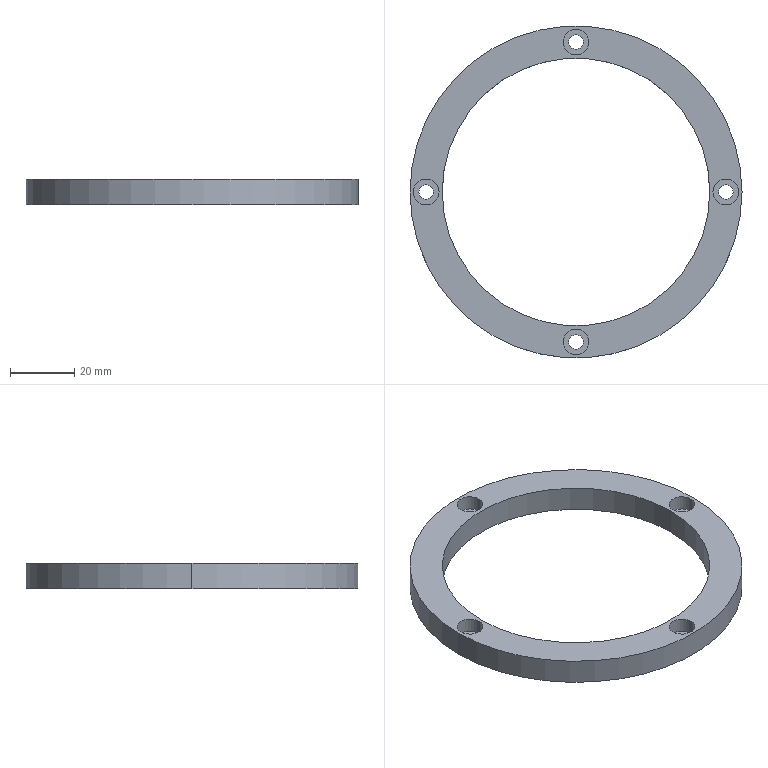Part | SolidWorks | features CirPattern 1, Extrusion 1, HoleWzd 1 | 1 solid | 26 faces | box 103 x 103 x 8 mm | volume 22232 mm3 | cylinder 20 | plane 6 | commonest cylinder face diameters 4.5 x8 8 x8 83 x2 103 x2
STEP:
#1=CARTESIAN_POINT('',(-50.5,0.,3.4));
#2=VERTEX_POINT('',#1);
#3=CARTESIAN_POINT('',(-42.5,0.,3.4));
#4=VERTEX_POINT('',#3);
#5=CARTESIAN_POINT('',(-46.5,0.,3.4));
#6=DIRECTION('',(0.,0.,1.));
#7=DIRECTION('',(1.,0.,0.));
#8=AXIS2_PLACEMENT_3D('',#5,#6,#7);
#9=CIRCLE('',#8,4.);
#10=EDGE_CURVE('',#2,#4,#9,.T.);
#11=ORIENTED_EDGE('',*,*,#10,.F.);
#12=CARTESIAN_POINT('',(-50.5,0.,8.));
#13=VERTEX_POINT('',#12);
#14=CARTESIAN_POINT('',(-50.5,0.,8.));
#15=DIRECTION('',(0.,0.,1.));
#16=VECTOR('',#15,1000.);
#17=LINE('',#14,#16);
#18=EDGE_CURVE('',#2,#13,#17,.T.);
#19=ORIENTED_EDGE('',*,*,#18,.T.);
#20=CARTESIAN_POINT('',(-42.5,0.,8.));
#21=VERTEX_POINT('',#20);
#22=CARTESIAN_POINT('',(-46.5,0.,8.));
#23=DIRECTION('',(0.,0.,1.));
#24=DIRECTION('',(1.,0.,0.));
#25=AXIS2_PLACEMENT_3D('',#22,#23,#24);
#26=CIRCLE('',#25,4.);
#27=EDGE_CURVE('',#13,#21,#26,.T.);
#28=ORIENTED_EDGE('',*,*,#27,.T.);
#29=CARTESIAN_POINT('',(-42.5,0.,8.));
#30=DIRECTION('',(0.,0.,1.));
#31=VECTOR('',#30,1000.);
#32=LINE('',#29,#31);
#33=EDGE_CURVE('',#4,#21,#32,.T.);
#34=ORIENTED_EDGE('',*,*,#33,.F.);
#35=EDGE_LOOP('',(#11,#19,#28,#34));
#36=FACE_OUTER_BOUND('',#35,.T.);
#37=CARTESIAN_POINT('',(-46.5,0.,8.));
#38=DIRECTION('',(0.,0.,1.));
#39=DIRECTION('',(1.,0.,0.));
#40=AXIS2_PLACEMENT_3D('',#37,#38,#39);
#41=CYLINDRICAL_SURFACE('',#40,4.);
#42=ADVANCED_FACE('',(#36),#41,.F.);
#43=CARTESIAN_POINT('',(-48.75,0.,0.));
#44=VERTEX_POINT('',#43);
#45=CARTESIAN_POINT('',(-44.25,0.,0.));
#46=VERTEX_POINT('',#45);
#47=CARTESIAN_POINT('',(-46.5,0.,0.));
#48=DIRECTION('',(0.,0.,1.));
#49=DIRECTION('',(1.,0.,0.));
#50=AXIS2_PLACEMENT_3D('',#47,#48,#49);
#51=CIRCLE('',#50,2.25);
#52=EDGE_CURVE('',#44,#46,#51,.T.);
#53=ORIENTED_EDGE('',*,*,#52,.F.);
#54=CARTESIAN_POINT('',(-48.75,0.,3.4));
#55=VERTEX_POINT('',#54);
#56=CARTESIAN_POINT('',(-48.75,0.,8.));
#57=DIRECTION('',(0.,0.,1.));
#58=VECTOR('',#57,1000.);
#59=LINE('',#56,#58);
#60=EDGE_CURVE('',#44,#55,#59,.T.);
#61=ORIENTED_EDGE('',*,*,#60,.T.);
#62=CARTESIAN_POINT('',(-44.25,0.,3.4));
#63=VERTEX_POINT('',#62);
#64=CARTESIAN_POINT('',(-46.5,0.,3.4));
#65=DIRECTION('',(0.,0.,1.));
#66=DIRECTION('',(1.,0.,0.));
#67=AXIS2_PLACEMENT_3D('',#64,#65,#66);
#68=CIRCLE('',#67,2.25);
#69=EDGE_CURVE('',#55,#63,#68,.T.);
#70=ORIENTED_EDGE('',*,*,#69,.T.);
#71=CARTESIAN_POINT('',(-44.25,0.,8.));
#72=DIRECTION('',(0.,0.,1.));
#73=VECTOR('',#72,1000.);
#74=LINE('',#71,#73);
#75=EDGE_CURVE('',#46,#63,#74,.T.);
#76=ORIENTED_EDGE('',*,*,#75,.F.);
#77=EDGE_LOOP('',(#53,#61,#70,#76));
#78=FACE_OUTER_BOUND('',#77,.T.);
#79=CARTESIAN_POINT('',(-46.5,0.,8.));
#80=DIRECTION('',(0.,0.,1.));
#81=DIRECTION('',(1.,0.,0.));
#82=AXIS2_PLACEMENT_3D('',#79,#80,#81);
#83=CYLINDRICAL_SURFACE('',#82,2.25);
#84=ADVANCED_FACE('',(#78),#83,.F.);
#85=CARTESIAN_POINT('',(-4.,-46.5,3.4));
#86=VERTEX_POINT('',#85);
#87=CARTESIAN_POINT('',(4.,-46.5,3.4));
#88=VERTEX_POINT('',#87);
#89=CARTESIAN_POINT('',(0.,-46.5,3.4));
#90=DIRECTION('',(0.,0.,1.));
#91=DIRECTION('',(1.,0.,0.));
#92=AXIS2_PLACEMENT_3D('',#89,#90,#91);
#93=CIRCLE('',#92,4.);
#94=EDGE_CURVE('',#86,#88,#93,.T.);
#95=ORIENTED_EDGE('',*,*,#94,.F.);
#96=CARTESIAN_POINT('',(-4.,-46.5,8.));
#97=VERTEX_POINT('',#96);
#98=CARTESIAN_POINT('',(-4.,-46.5,8.));
#99=DIRECTION('',(0.,0.,1.));
#100=VECTOR('',#99,1000.);
#101=LINE('',#98,#100);
#102=EDGE_CURVE('',#86,#97,#101,.T.);
#103=ORIENTED_EDGE('',*,*,#102,.T.);
#104=CARTESIAN_POINT('',(4.,-46.5,8.));
#105=VERTEX_POINT('',#104);
#106=CARTESIAN_POINT('',(0.,-46.5,8.));
#107=DIRECTION('',(0.,0.,1.));
#108=DIRECTION('',(1.,0.,0.));
#109=AXIS2_PLACEMENT_3D('',#106,#107,#108);
#110=CIRCLE('',#109,4.);
#111=EDGE_CURVE('',#97,#105,#110,.T.);
#112=ORIENTED_EDGE('',*,*,#111,.T.);
#113=CARTESIAN_POINT('',(4.,-46.5,8.));
#114=DIRECTION('',(0.,0.,1.));
#115=VECTOR('',#114,1000.);
#116=LINE('',#113,#115);
#117=EDGE_CURVE('',#88,#105,#116,.T.);
#118=ORIENTED_EDGE('',*,*,#117,.F.);
#119=EDGE_LOOP('',(#95,#103,#112,#118));
#120=FACE_OUTER_BOUND('',#119,.T.);
#121=CARTESIAN_POINT('',(0.,-46.5,8.));
#122=DIRECTION('',(0.,0.,1.));
#123=DIRECTION('',(1.,0.,0.));
#124=AXIS2_PLACEMENT_3D('',#121,#122,#123);
#125=CYLINDRICAL_SURFACE('',#124,4.);
#126=ADVANCED_FACE('',(#120),#125,.F.);
#127=CARTESIAN_POINT('',(-2.25,-46.5,0.));
#128=VERTEX_POINT('',#127);
#129=CARTESIAN_POINT('',(2.25,-46.5,0.));
#130=VERTEX_POINT('',#129);
#131=CARTESIAN_POINT('',(0.,-46.5,0.));
#132=DIRECTION('',(0.,0.,1.));
#133=DIRECTION('',(1.,0.,0.));
#134=AXIS2_PLACEMENT_3D('',#131,#132,#133);
#135=CIRCLE('',#134,2.25);
#136=EDGE_CURVE('',#128,#130,#135,.T.);
#137=ORIENTED_EDGE('',*,*,#136,.F.);
#138=CARTESIAN_POINT('',(-2.25,-46.5,3.4));
#139=VERTEX_POINT('',#138);
#140=CARTESIAN_POINT('',(-2.25,-46.5,8.));
#141=DIRECTION('',(0.,0.,1.));
#142=VECTOR('',#141,1000.);
#143=LINE('',#140,#142);
#144=EDGE_CURVE('',#128,#139,#143,.T.);
#145=ORIENTED_EDGE('',*,*,#144,.T.);
#146=CARTESIAN_POINT('',(2.25,-46.5,3.4));
#147=VERTEX_POINT('',#146);
#148=CARTESIAN_POINT('',(0.,-46.5,3.4));
#149=DIRECTION('',(0.,0.,1.));
#150=DIRECTION('',(1.,0.,0.));
#151=AXIS2_PLACEMENT_3D('',#148,#149,#150);
#152=CIRCLE('',#151,2.25);
#153=EDGE_CURVE('',#139,#147,#152,.T.);
#154=ORIENTED_EDGE('',*,*,#153,.T.);
#155=CARTESIAN_POINT('',(2.25,-46.5,8.));
#156=DIRECTION('',(0.,0.,1.));
#157=VECTOR('',#156,1000.);
#158=LINE('',#155,#157);
#159=EDGE_CURVE('',#130,#147,#158,.T.);
#160=ORIENTED_EDGE('',*,*,#159,.F.);
#161=EDGE_LOOP('',(#137,#145,#154,#160));
#162=FACE_OUTER_BOUND('',#161,.T.);
#163=CARTESIAN_POINT('',(0.,-46.5,8.));
#164=DIRECTION('',(0.,0.,1.));
#165=DIRECTION('',(1.,0.,0.));
#166=AXIS2_PLACEMENT_3D('',#163,#164,#165);
#167=CYLINDRICAL_SURFACE('',#166,2.25);
#168=ADVANCED_FACE('',(#162),#167,.F.);
#169=CARTESIAN_POINT('',(42.5,0.,3.4));
#170=VERTEX_POINT('',#169);
#171=CARTESIAN_POINT('',(50.5,0.,3.4));
#172=VERTEX_POINT('',#171);
#173=CARTESIAN_POINT('',(46.5,0.,3.4));
#174=DIRECTION('',(0.,0.,1.));
#175=DIRECTION('',(1.,0.,0.));
#176=AXIS2_PLACEMENT_3D('',#173,#174,#175);
#177=CIRCLE('',#176,4.);
#178=EDGE_CURVE('',#170,#172,#177,.T.);
#179=ORIENTED_EDGE('',*,*,#178,.F.);
#180=CARTESIAN_POINT('',(42.5,0.,8.));
#181=VERTEX_POINT('',#180);
#182=CARTESIAN_POINT('',(42.5,0.,8.));
#183=DIRECTION('',(0.,0.,1.));
#184=VECTOR('',#183,1000.);
#185=LINE('',#182,#184);
#186=EDGE_CURVE('',#170,#181,#185,.T.);
#187=ORIENTED_EDGE('',*,*,#186,.T.);
#188=CARTESIAN_POINT('',(50.5,0.,8.));
#189=VERTEX_POINT('',#188);
#190=CARTESIAN_POINT('',(46.5,0.,8.));
#191=DIRECTION('',(0.,0.,1.));
#192=DIRECTION('',(1.,0.,0.));
#193=AXIS2_PLACEMENT_3D('',#190,#191,#192);
#194=CIRCLE('',#193,4.);
#195=EDGE_CURVE('',#181,#189,#194,.T.);
#196=ORIENTED_EDGE('',*,*,#195,.T.);
#197=CARTESIAN_POINT('',(50.5,0.,8.));
#198=DIRECTION('',(0.,0.,1.));
#199=VECTOR('',#198,1000.);
#200=LINE('',#197,#199);
#201=EDGE_CURVE('',#172,#189,#200,.T.);
#202=ORIENTED_EDGE('',*,*,#201,.F.);
#203=EDGE_LOOP('',(#179,#187,#196,#202));
#204=FACE_OUTER_BOUND('',#203,.T.);
#205=CARTESIAN_POINT('',(46.5,0.,8.));
#206=DIRECTION('',(0.,0.,1.));
#207=DIRECTION('',(1.,0.,0.));
#208=AXIS2_PLACEMENT_3D('',#205,#206,#207);
#209=CYLINDRICAL_SURFACE('',#208,4.);
#210=ADVANCED_FACE('',(#204),#209,.F.);
#211=CARTESIAN_POINT('',(44.25,0.,0.));
#212=VERTEX_POINT('',#211);
#213=CARTESIAN_POINT('',(48.75,0.,0.));
#214=VERTEX_POINT('',#213);
#215=CARTESIAN_POINT('',(46.5,0.,0.));
#216=DIRECTION('',(0.,0.,1.));
#217=DIRECTION('',(1.,0.,0.));
#218=AXIS2_PLACEMENT_3D('',#215,#216,#217);
#219=CIRCLE('',#218,2.25);
#220=EDGE_CURVE('',#212,#214,#219,.T.);
#221=ORIENTED_EDGE('',*,*,#220,.F.);
#222=CARTESIAN_POINT('',(44.25,0.,3.4));
#223=VERTEX_POINT('',#222);
#224=CARTESIAN_POINT('',(44.25,0.,8.));
#225=DIRECTION('',(0.,0.,1.));
#226=VECTOR('',#225,1000.);
#227=LINE('',#224,#226);
#228=EDGE_CURVE('',#212,#223,#227,.T.);
#229=ORIENTED_EDGE('',*,*,#228,.T.);
#230=CARTESIAN_POINT('',(48.75,0.,3.4));
#231=VERTEX_POINT('',#230);
#232=CARTESIAN_POINT('',(46.5,0.,3.4));
#233=DIRECTION('',(0.,0.,1.));
#234=DIRECTION('',(1.,0.,0.));
#235=AXIS2_PLACEMENT_3D('',#232,#233,#234);
#236=CIRCLE('',#235,2.25);
#237=EDGE_CURVE('',#223,#231,#236,.T.);
#238=ORIENTED_EDGE('',*,*,#237,.T.);
#239=CARTESIAN_POINT('',(48.75,0.,8.));
#240=DIRECTION('',(0.,0.,1.));
#241=VECTOR('',#240,1000.);
#242=LINE('',#239,#241);
#243=EDGE_CURVE('',#214,#231,#242,.T.);
#244=ORIENTED_EDGE('',*,*,#243,.F.);
#245=EDGE_LOOP('',(#221,#229,#238,#244));
#246=FACE_OUTER_BOUND('',#245,.T.);
#247=CARTESIAN_POINT('',(46.5,0.,8.));
#248=DIRECTION('',(0.,0.,1.));
#249=DIRECTION('',(1.,0.,0.));
#250=AXIS2_PLACEMENT_3D('',#247,#248,#249);
#251=CYLINDRICAL_SURFACE('',#250,2.25);
#252=ADVANCED_FACE('',(#246),#251,.F.);
#253=CARTESIAN_POINT('',(-4.,46.5,3.4));
#254=VERTEX_POINT('',#253);
#255=CARTESIAN_POINT('',(4.,46.5,3.4));
#256=VERTEX_POINT('',#255);
#257=CARTESIAN_POINT('',(0.,46.5,3.4));
#258=DIRECTION('',(0.,0.,1.));
#259=DIRECTION('',(1.,0.,0.));
#260=AXIS2_PLACEMENT_3D('',#257,#258,#259);
#261=CIRCLE('',#260,4.);
#262=EDGE_CURVE('',#254,#256,#261,.T.);
#263=ORIENTED_EDGE('',*,*,#262,.F.);
#264=CARTESIAN_POINT('',(-4.,46.5,8.));
#265=VERTEX_POINT('',#264);
#266=CARTESIAN_POINT('',(-4.,46.5,8.));
#267=DIRECTION('',(0.,0.,1.));
#268=VECTOR('',#267,1000.);
#269=LINE('',#266,#268);
#270=EDGE_CURVE('',#254,#265,#269,.T.);
#271=ORIENTED_EDGE('',*,*,#270,.T.);
#272=CARTESIAN_POINT('',(4.,46.5,8.));
#273=VERTEX_POINT('',#272);
#274=CARTESIAN_POINT('',(0.,46.5,8.));
#275=DIRECTION('',(0.,0.,1.));
#276=DIRECTION('',(1.,0.,0.));
#277=AXIS2_PLACEMENT_3D('',#274,#275,#276);
#278=CIRCLE('',#277,4.);
#279=EDGE_CURVE('',#265,#273,#278,.T.);
#280=ORIENTED_EDGE('',*,*,#279,.T.);
#281=CARTESIAN_POINT('',(4.,46.5,8.));
#282=DIRECTION('',(0.,0.,1.));
#283=VECTOR('',#282,1000.);
#284=LINE('',#281,#283);
#285=EDGE_CURVE('',#256,#273,#284,.T.);
#286=ORIENTED_EDGE('',*,*,#285,.F.);
#287=EDGE_LOOP('',(#263,#271,#280,#286));
#288=FACE_OUTER_BOUND('',#287,.T.);
#289=CARTESIAN_POINT('',(0.,46.5,8.));
#290=DIRECTION('',(0.,0.,1.));
#291=DIRECTION('',(1.,0.,0.));
#292=AXIS2_PLACEMENT_3D('',#289,#290,#291);
#293=CYLINDRICAL_SURFACE('',#292,4.);
#294=ADVANCED_FACE('',(#288),#293,.F.);
#295=CARTESIAN_POINT('',(-2.25,46.5,0.));
#296=VERTEX_POINT('',#295);
#297=CARTESIAN_POINT('',(2.25,46.5,0.));
#298=VERTEX_POINT('',#297);
#299=CARTESIAN_POINT('',(0.,46.5,0.));
#300=DIRECTION('',(0.,0.,1.));
#301=DIRECTION('',(1.,0.,0.));
#302=AXIS2_PLACEMENT_3D('',#299,#300,#301);
#303=CIRCLE('',#302,2.25);
#304=EDGE_CURVE('',#296,#298,#303,.T.);
#305=ORIENTED_EDGE('',*,*,#304,.F.);
#306=CARTESIAN_POINT('',(-2.25,46.5,3.4));
#307=VERTEX_POINT('',#306);
#308=CARTESIAN_POINT('',(-2.25,46.5,8.));
#309=DIRECTION('',(0.,0.,1.));
#310=VECTOR('',#309,1000.);
#311=LINE('',#308,#310);
#312=EDGE_CURVE('',#296,#307,#311,.T.);
#313=ORIENTED_EDGE('',*,*,#312,.T.);
#314=CARTESIAN_POINT('',(2.25,46.5,3.4));
#315=VERTEX_POINT('',#314);
#316=CARTESIAN_POINT('',(0.,46.5,3.4));
#317=DIRECTION('',(0.,0.,1.));
#318=DIRECTION('',(1.,0.,0.));
#319=AXIS2_PLACEMENT_3D('',#316,#317,#318);
#320=CIRCLE('',#319,2.25);
#321=EDGE_CURVE('',#307,#315,#320,.T.);
#322=ORIENTED_EDGE('',*,*,#321,.T.);
#323=CARTESIAN_POINT('',(2.25,46.5,8.));
#324=DIRECTION('',(0.,0.,1.));
#325=VECTOR('',#324,1000.);
#326=LINE('',#323,#325);
#327=EDGE_CURVE('',#298,#315,#326,.T.);
#328=ORIENTED_EDGE('',*,*,#327,.F.);
#329=EDGE_LOOP('',(#305,#313,#322,#328));
#330=FACE_OUTER_BOUND('',#329,.T.);
#331=CARTESIAN_POINT('',(0.,46.5,8.));
#332=DIRECTION('',(0.,0.,1.));
#333=DIRECTION('',(1.,0.,0.));
#334=AXIS2_PLACEMENT_3D('',#331,#332,#333);
#335=CYLINDRICAL_SURFACE('',#334,2.25);
#336=ADVANCED_FACE('',(#330),#335,.F.);
#337=CARTESIAN_POINT('',(-41.5,0.,8.));
#338=VERTEX_POINT('',#337);
#339=CARTESIAN_POINT('',(41.5,0.,8.));
#340=VERTEX_POINT('',#339);
#341=CARTESIAN_POINT('',(0.,0.,8.));
#342=DIRECTION('',(0.,0.,1.));
#343=DIRECTION('',(1.,0.,0.));
#344=AXIS2_PLACEMENT_3D('',#341,#342,#343);
#345=CIRCLE('',#344,41.5);
#346=EDGE_CURVE('',#338,#340,#345,.T.);
#347=ORIENTED_EDGE('',*,*,#346,.T.);
#348=CARTESIAN_POINT('',(41.5,0.,0.));
#349=VERTEX_POINT('',#348);
#350=CARTESIAN_POINT('',(41.5,0.,8.));
#351=DIRECTION('',(0.,0.,-1.));
#352=VECTOR('',#351,1000.);
#353=LINE('',#350,#352);
#354=EDGE_CURVE('',#340,#349,#353,.T.);
#355=ORIENTED_EDGE('',*,*,#354,.T.);
#356=CARTESIAN_POINT('',(-41.5,0.,0.));
#357=VERTEX_POINT('',#356);
#358=CARTESIAN_POINT('',(0.,0.,0.));
#359=DIRECTION('',(0.,0.,1.));
#360=DIRECTION('',(1.,0.,0.));
#361=AXIS2_PLACEMENT_3D('',#358,#359,#360);
#362=CIRCLE('',#361,41.5);
#363=EDGE_CURVE('',#357,#349,#362,.T.);
#364=ORIENTED_EDGE('',*,*,#363,.F.);
#365=CARTESIAN_POINT('',(-41.5,0.,8.));
#366=DIRECTION('',(0.,0.,-1.));
#367=VECTOR('',#366,1000.);
#368=LINE('',#365,#367);
#369=EDGE_CURVE('',#338,#357,#368,.T.);
#370=ORIENTED_EDGE('',*,*,#369,.F.);
#371=EDGE_LOOP('',(#347,#355,#364,#370));
#372=FACE_OUTER_BOUND('',#371,.T.);
#373=CARTESIAN_POINT('',(0.,0.,8.));
#374=DIRECTION('',(0.,0.,-1.));
#375=DIRECTION('',(-1.,0.,0.));
#376=AXIS2_PLACEMENT_3D('',#373,#374,#375);
#377=CYLINDRICAL_SURFACE('',#376,41.5);
#378=ADVANCED_FACE('',(#372),#377,.F.);
#379=CARTESIAN_POINT('',(51.5,0.,8.));
#380=VERTEX_POINT('',#379);
#381=CARTESIAN_POINT('',(-51.5,0.,8.));
#382=VERTEX_POINT('',#381);
#383=CARTESIAN_POINT('',(0.,0.,8.));
#384=DIRECTION('',(0.,0.,1.));
#385=DIRECTION('',(1.,0.,0.));
#386=AXIS2_PLACEMENT_3D('',#383,#384,#385);
#387=CIRCLE('',#386,51.5);
#388=EDGE_CURVE('',#380,#382,#387,.T.);
#389=ORIENTED_EDGE('',*,*,#388,.F.);
#390=CARTESIAN_POINT('',(51.5,0.,0.));
#391=VERTEX_POINT('',#390);
#392=CARTESIAN_POINT('',(51.5,0.,8.));
#393=DIRECTION('',(0.,0.,-1.));
#394=VECTOR('',#393,1000.);
#395=LINE('',#392,#394);
#396=EDGE_CURVE('',#380,#391,#395,.T.);
#397=ORIENTED_EDGE('',*,*,#396,.T.);
#398=CARTESIAN_POINT('',(-51.5,0.,0.));
#399=VERTEX_POINT('',#398);
#400=CARTESIAN_POINT('',(0.,0.,0.));
#401=DIRECTION('',(0.,0.,1.));
#402=DIRECTION('',(1.,0.,0.));
#403=AXIS2_PLACEMENT_3D('',#400,#401,#402);
#404=CIRCLE('',#403,51.5);
#405=EDGE_CURVE('',#391,#399,#404,.T.);
#406=ORIENTED_EDGE('',*,*,#405,.T.);
#407=CARTESIAN_POINT('',(-51.5,0.,8.));
#408=DIRECTION('',(0.,0.,-1.));
#409=VECTOR('',#408,1000.);
#410=LINE('',#407,#409);
#411=EDGE_CURVE('',#382,#399,#410,.T.);
#412=ORIENTED_EDGE('',*,*,#411,.F.);
#413=EDGE_LOOP('',(#389,#397,#406,#412));
#414=FACE_OUTER_BOUND('',#413,.T.);
#415=CARTESIAN_POINT('',(0.,0.,8.));
#416=DIRECTION('',(0.,0.,-1.));
#417=DIRECTION('',(-1.,0.,0.));
#418=AXIS2_PLACEMENT_3D('',#415,#416,#417);
#419=CYLINDRICAL_SURFACE('',#418,51.5);
#420=ADVANCED_FACE('',(#414),#419,.T.);
#421=CARTESIAN_POINT('',(-46.5,0.,8.));
#422=DIRECTION('',(0.,0.,1.));
#423=DIRECTION('',(1.,0.,0.));
#424=AXIS2_PLACEMENT_3D('',#421,#422,#423);
#425=CIRCLE('',#424,4.);
#426=EDGE_CURVE('',#21,#13,#425,.T.);
#427=ORIENTED_EDGE('',*,*,#426,.F.);
#428=ORIENTED_EDGE('',*,*,#27,.F.);
#429=EDGE_LOOP('',(#427,#428));
#430=FACE_BOUND('',#429,.T.);
#431=CARTESIAN_POINT('',(0.,-46.5,8.));
#432=DIRECTION('',(0.,0.,1.));
#433=DIRECTION('',(1.,0.,0.));
#434=AXIS2_PLACEMENT_3D('',#431,#432,#433);
#435=CIRCLE('',#434,4.);
#436=EDGE_CURVE('',#105,#97,#435,.T.);
#437=ORIENTED_EDGE('',*,*,#436,.F.);
#438=ORIENTED_EDGE('',*,*,#111,.F.);
#439=EDGE_LOOP('',(#437,#438));
#440=FACE_BOUND('',#439,.T.);
#441=CARTESIAN_POINT('',(46.5,0.,8.));
#442=DIRECTION('',(0.,0.,1.));
#443=DIRECTION('',(1.,0.,0.));
#444=AXIS2_PLACEMENT_3D('',#441,#442,#443);
#445=CIRCLE('',#444,4.);
#446=EDGE_CURVE('',#189,#181,#445,.T.);
#447=ORIENTED_EDGE('',*,*,#446,.F.);
#448=ORIENTED_EDGE('',*,*,#195,.F.);
#449=EDGE_LOOP('',(#447,#448));
#450=FACE_BOUND('',#449,.T.);
#451=CARTESIAN_POINT('',(0.,46.5,8.));
#452=DIRECTION('',(0.,0.,1.));
#453=DIRECTION('',(1.,0.,0.));
#454=AXIS2_PLACEMENT_3D('',#451,#452,#453);
#455=CIRCLE('',#454,4.);
#456=EDGE_CURVE('',#273,#265,#455,.T.);
#457=ORIENTED_EDGE('',*,*,#456,.F.);
#458=ORIENTED_EDGE('',*,*,#279,.F.);
#459=EDGE_LOOP('',(#457,#458));
#460=FACE_BOUND('',#459,.T.);
#461=CARTESIAN_POINT('',(0.,0.,8.));
#462=DIRECTION('',(0.,0.,1.));
#463=DIRECTION('',(1.,0.,0.));
#464=AXIS2_PLACEMENT_3D('',#461,#462,#463);
#465=CIRCLE('',#464,51.5);
#466=EDGE_CURVE('',#382,#380,#465,.T.);
#467=ORIENTED_EDGE('',*,*,#466,.T.);
#468=ORIENTED_EDGE('',*,*,#388,.T.);
#469=EDGE_LOOP('',(#467,#468));
#470=FACE_OUTER_BOUND('',#469,.T.);
#471=ORIENTED_EDGE('',*,*,#346,.F.);
#472=CARTESIAN_POINT('',(0.,0.,8.));
#473=DIRECTION('',(0.,0.,1.));
#474=DIRECTION('',(1.,0.,0.));
#475=AXIS2_PLACEMENT_3D('',#472,#473,#474);
#476=CIRCLE('',#475,41.5);
#477=EDGE_CURVE('',#340,#338,#476,.T.);
#478=ORIENTED_EDGE('',*,*,#477,.F.);
#479=EDGE_LOOP('',(#471,#478));
#480=FACE_BOUND('',#479,.T.);
#481=CARTESIAN_POINT('',(0.,0.,8.));
#482=DIRECTION('',(0.,0.,1.));
#483=DIRECTION('',(1.,0.,0.));
#484=AXIS2_PLACEMENT_3D('',#481,#482,#483);
#485=PLANE('',#484);
#486=ADVANCED_FACE('',(#430,#440,#450,#460,#470,#480),#485,.T.);
#487=CARTESIAN_POINT('',(-46.5,0.,0.));
#488=DIRECTION('',(0.,0.,1.));
#489=DIRECTION('',(1.,0.,0.));
#490=AXIS2_PLACEMENT_3D('',#487,#488,#489);
#491=CIRCLE('',#490,2.25);
#492=EDGE_CURVE('',#46,#44,#491,.T.);
#493=ORIENTED_EDGE('',*,*,#492,.T.);
#494=ORIENTED_EDGE('',*,*,#52,.T.);
#495=EDGE_LOOP('',(#493,#494));
#496=FACE_BOUND('',#495,.T.);
#497=CARTESIAN_POINT('',(0.,-46.5,0.));
#498=DIRECTION('',(0.,0.,1.));
#499=DIRECTION('',(1.,0.,0.));
#500=AXIS2_PLACEMENT_3D('',#497,#498,#499);
#501=CIRCLE('',#500,2.25);
#502=EDGE_CURVE('',#130,#128,#501,.T.);
#503=ORIENTED_EDGE('',*,*,#502,.T.);
#504=ORIENTED_EDGE('',*,*,#136,.T.);
#505=EDGE_LOOP('',(#503,#504));
#506=FACE_BOUND('',#505,.T.);
#507=CARTESIAN_POINT('',(46.5,0.,0.));
#508=DIRECTION('',(0.,0.,1.));
#509=DIRECTION('',(1.,0.,0.));
#510=AXIS2_PLACEMENT_3D('',#507,#508,#509);
#511=CIRCLE('',#510,2.25);
#512=EDGE_CURVE('',#214,#212,#511,.T.);
#513=ORIENTED_EDGE('',*,*,#512,.T.);
#514=ORIENTED_EDGE('',*,*,#220,.T.);
#515=EDGE_LOOP('',(#513,#514));
#516=FACE_BOUND('',#515,.T.);
#517=CARTESIAN_POINT('',(0.,46.5,0.));
#518=DIRECTION('',(0.,0.,1.));
#519=DIRECTION('',(1.,0.,0.));
#520=AXIS2_PLACEMENT_3D('',#517,#518,#519);
#521=CIRCLE('',#520,2.25);
#522=EDGE_CURVE('',#298,#296,#521,.T.);
#523=ORIENTED_EDGE('',*,*,#522,.T.);
#524=ORIENTED_EDGE('',*,*,#304,.T.);
#525=EDGE_LOOP('',(#523,#524));
#526=FACE_BOUND('',#525,.T.);
#527=CARTESIAN_POINT('',(0.,0.,0.));
#528=DIRECTION('',(0.,0.,1.));
#529=DIRECTION('',(1.,0.,0.));
#530=AXIS2_PLACEMENT_3D('',#527,#528,#529);
#531=CIRCLE('',#530,51.5);
#532=EDGE_CURVE('',#399,#391,#531,.T.);
#533=ORIENTED_EDGE('',*,*,#532,.F.);
#534=ORIENTED_EDGE('',*,*,#405,.F.);
#535=EDGE_LOOP('',(#533,#534));
#536=FACE_OUTER_BOUND('',#535,.T.);
#537=ORIENTED_EDGE('',*,*,#363,.T.);
#538=CARTESIAN_POINT('',(0.,0.,0.));
#539=DIRECTION('',(0.,0.,1.));
#540=DIRECTION('',(1.,0.,0.));
#541=AXIS2_PLACEMENT_3D('',#538,#539,#540);
#542=CIRCLE('',#541,41.5);
#543=EDGE_CURVE('',#349,#357,#542,.T.);
#544=ORIENTED_EDGE('',*,*,#543,.T.);
#545=EDGE_LOOP('',(#537,#544));
#546=FACE_BOUND('',#545,.T.);
#547=CARTESIAN_POINT('',(0.,0.,0.));
#548=DIRECTION('',(0.,0.,1.));
#549=DIRECTION('',(1.,0.,0.));
#550=AXIS2_PLACEMENT_3D('',#547,#548,#549);
#551=PLANE('',#550);
#552=ADVANCED_FACE('',(#496,#506,#516,#526,#536,#546),#551,.F.);
#553=ORIENTED_EDGE('',*,*,#396,.F.);
#554=ORIENTED_EDGE('',*,*,#466,.F.);
#555=ORIENTED_EDGE('',*,*,#411,.T.);
#556=ORIENTED_EDGE('',*,*,#532,.T.);
#557=EDGE_LOOP('',(#553,#554,#555,#556));
#558=FACE_OUTER_BOUND('',#557,.T.);
#559=CARTESIAN_POINT('',(0.,0.,8.));
#560=DIRECTION('',(0.,0.,-1.));
#561=DIRECTION('',(-1.,0.,0.));
#562=AXIS2_PLACEMENT_3D('',#559,#560,#561);
#563=CYLINDRICAL_SURFACE('',#562,51.5);
#564=ADVANCED_FACE('',(#558),#563,.T.);
#565=ORIENTED_EDGE('',*,*,#354,.F.);
#566=ORIENTED_EDGE('',*,*,#477,.T.);
#567=ORIENTED_EDGE('',*,*,#369,.T.);
#568=ORIENTED_EDGE('',*,*,#543,.F.);
#569=EDGE_LOOP('',(#565,#566,#567,#568));
#570=FACE_OUTER_BOUND('',#569,.T.);
#571=CARTESIAN_POINT('',(0.,0.,8.));
#572=DIRECTION('',(0.,0.,-1.));
#573=DIRECTION('',(-1.,0.,0.));
#574=AXIS2_PLACEMENT_3D('',#571,#572,#573);
#575=CYLINDRICAL_SURFACE('',#574,41.5);
#576=ADVANCED_FACE('',(#570),#575,.F.);
#577=ORIENTED_EDGE('',*,*,#312,.F.);
#578=ORIENTED_EDGE('',*,*,#522,.F.);
#579=ORIENTED_EDGE('',*,*,#327,.T.);
#580=CARTESIAN_POINT('',(0.,46.5,3.4));
#581=DIRECTION('',(0.,0.,1.));
#582=DIRECTION('',(1.,0.,0.));
#583=AXIS2_PLACEMENT_3D('',#580,#581,#582);
#584=CIRCLE('',#583,2.25);
#585=EDGE_CURVE('',#315,#307,#584,.T.);
#586=ORIENTED_EDGE('',*,*,#585,.T.);
#587=EDGE_LOOP('',(#577,#578,#579,#586));
#588=FACE_OUTER_BOUND('',#587,.T.);
#589=CARTESIAN_POINT('',(0.,46.5,8.));
#590=DIRECTION('',(0.,0.,1.));
#591=DIRECTION('',(1.,0.,0.));
#592=AXIS2_PLACEMENT_3D('',#589,#590,#591);
#593=CYLINDRICAL_SURFACE('',#592,2.25);
#594=ADVANCED_FACE('',(#588),#593,.F.);
#595=ORIENTED_EDGE('',*,*,#585,.F.);
#596=ORIENTED_EDGE('',*,*,#321,.F.);
#597=EDGE_LOOP('',(#595,#596));
#598=FACE_BOUND('',#597,.T.);
#599=CARTESIAN_POINT('',(0.,46.5,3.4));
#600=DIRECTION('',(0.,0.,1.));
#601=DIRECTION('',(1.,0.,0.));
#602=AXIS2_PLACEMENT_3D('',#599,#600,#601);
#603=CIRCLE('',#602,4.);
#604=EDGE_CURVE('',#256,#254,#603,.T.);
#605=ORIENTED_EDGE('',*,*,#604,.T.);
#606=ORIENTED_EDGE('',*,*,#262,.T.);
#607=EDGE_LOOP('',(#605,#606));
#608=FACE_OUTER_BOUND('',#607,.T.);
#609=CARTESIAN_POINT('',(2.25,46.5,3.4));
#610=DIRECTION('',(0.,0.,-1.));
#611=DIRECTION('',(-1.,0.,0.));
#612=AXIS2_PLACEMENT_3D('',#609,#610,#611);
#613=PLANE('',#612);
#614=ADVANCED_FACE('',(#598,#608),#613,.F.);
#615=ORIENTED_EDGE('',*,*,#270,.F.);
#616=ORIENTED_EDGE('',*,*,#604,.F.);
#617=ORIENTED_EDGE('',*,*,#285,.T.);
#618=ORIENTED_EDGE('',*,*,#456,.T.);
#619=EDGE_LOOP('',(#615,#616,#617,#618));
#620=FACE_OUTER_BOUND('',#619,.T.);
#621=CARTESIAN_POINT('',(0.,46.5,8.));
#622=DIRECTION('',(0.,0.,1.));
#623=DIRECTION('',(1.,0.,0.));
#624=AXIS2_PLACEMENT_3D('',#621,#622,#623);
#625=CYLINDRICAL_SURFACE('',#624,4.);
#626=ADVANCED_FACE('',(#620),#625,.F.);
#627=ORIENTED_EDGE('',*,*,#228,.F.);
#628=ORIENTED_EDGE('',*,*,#512,.F.);
#629=ORIENTED_EDGE('',*,*,#243,.T.);
#630=CARTESIAN_POINT('',(46.5,0.,3.4));
#631=DIRECTION('',(0.,0.,1.));
#632=DIRECTION('',(1.,0.,0.));
#633=AXIS2_PLACEMENT_3D('',#630,#631,#632);
#634=CIRCLE('',#633,2.25);
#635=EDGE_CURVE('',#231,#223,#634,.T.);
#636=ORIENTED_EDGE('',*,*,#635,.T.);
#637=EDGE_LOOP('',(#627,#628,#629,#636));
#638=FACE_OUTER_BOUND('',#637,.T.);
#639=CARTESIAN_POINT('',(46.5,0.,8.));
#640=DIRECTION('',(0.,0.,1.));
#641=DIRECTION('',(1.,0.,0.));
#642=AXIS2_PLACEMENT_3D('',#639,#640,#641);
#643=CYLINDRICAL_SURFACE('',#642,2.25);
#644=ADVANCED_FACE('',(#638),#643,.F.);
#645=ORIENTED_EDGE('',*,*,#635,.F.);
#646=ORIENTED_EDGE('',*,*,#237,.F.);
#647=EDGE_LOOP('',(#645,#646));
#648=FACE_BOUND('',#647,.T.);
#649=CARTESIAN_POINT('',(46.5,0.,3.4));
#650=DIRECTION('',(0.,0.,1.));
#651=DIRECTION('',(1.,0.,0.));
#652=AXIS2_PLACEMENT_3D('',#649,#650,#651);
#653=CIRCLE('',#652,4.);
#654=EDGE_CURVE('',#172,#170,#653,.T.);
#655=ORIENTED_EDGE('',*,*,#654,.T.);
#656=ORIENTED_EDGE('',*,*,#178,.T.);
#657=EDGE_LOOP('',(#655,#656));
#658=FACE_OUTER_BOUND('',#657,.T.);
#659=CARTESIAN_POINT('',(48.75,0.,3.4));
#660=DIRECTION('',(0.,0.,-1.));
#661=DIRECTION('',(-1.,0.,0.));
#662=AXIS2_PLACEMENT_3D('',#659,#660,#661);
#663=PLANE('',#662);
#664=ADVANCED_FACE('',(#648,#658),#663,.F.);
#665=ORIENTED_EDGE('',*,*,#186,.F.);
#666=ORIENTED_EDGE('',*,*,#654,.F.);
#667=ORIENTED_EDGE('',*,*,#201,.T.);
#668=ORIENTED_EDGE('',*,*,#446,.T.);
#669=EDGE_LOOP('',(#665,#666,#667,#668));
#670=FACE_OUTER_BOUND('',#669,.T.);
#671=CARTESIAN_POINT('',(46.5,0.,8.));
#672=DIRECTION('',(0.,0.,1.));
#673=DIRECTION('',(1.,0.,0.));
#674=AXIS2_PLACEMENT_3D('',#671,#672,#673);
#675=CYLINDRICAL_SURFACE('',#674,4.);
#676=ADVANCED_FACE('',(#670),#675,.F.);
#677=ORIENTED_EDGE('',*,*,#144,.F.);
#678=ORIENTED_EDGE('',*,*,#502,.F.);
#679=ORIENTED_EDGE('',*,*,#159,.T.);
#680=CARTESIAN_POINT('',(0.,-46.5,3.4));
#681=DIRECTION('',(0.,0.,1.));
#682=DIRECTION('',(1.,0.,0.));
#683=AXIS2_PLACEMENT_3D('',#680,#681,#682);
#684=CIRCLE('',#683,2.25);
#685=EDGE_CURVE('',#147,#139,#684,.T.);
#686=ORIENTED_EDGE('',*,*,#685,.T.);
#687=EDGE_LOOP('',(#677,#678,#679,#686));
#688=FACE_OUTER_BOUND('',#687,.T.);
#689=CARTESIAN_POINT('',(0.,-46.5,8.));
#690=DIRECTION('',(0.,0.,1.));
#691=DIRECTION('',(1.,0.,0.));
#692=AXIS2_PLACEMENT_3D('',#689,#690,#691);
#693=CYLINDRICAL_SURFACE('',#692,2.25);
#694=ADVANCED_FACE('',(#688),#693,.F.);
#695=ORIENTED_EDGE('',*,*,#685,.F.);
#696=ORIENTED_EDGE('',*,*,#153,.F.);
#697=EDGE_LOOP('',(#695,#696));
#698=FACE_BOUND('',#697,.T.);
#699=CARTESIAN_POINT('',(0.,-46.5,3.4));
#700=DIRECTION('',(0.,0.,1.));
#701=DIRECTION('',(1.,0.,0.));
#702=AXIS2_PLACEMENT_3D('',#699,#700,#701);
#703=CIRCLE('',#702,4.);
#704=EDGE_CURVE('',#88,#86,#703,.T.);
#705=ORIENTED_EDGE('',*,*,#704,.T.);
#706=ORIENTED_EDGE('',*,*,#94,.T.);
#707=EDGE_LOOP('',(#705,#706));
#708=FACE_OUTER_BOUND('',#707,.T.);
#709=CARTESIAN_POINT('',(2.25,-46.5,3.4));
#710=DIRECTION('',(0.,0.,-1.));
#711=DIRECTION('',(-1.,0.,0.));
#712=AXIS2_PLACEMENT_3D('',#709,#710,#711);
#713=PLANE('',#712);
#714=ADVANCED_FACE('',(#698,#708),#713,.F.);
#715=ORIENTED_EDGE('',*,*,#102,.F.);
#716=ORIENTED_EDGE('',*,*,#704,.F.);
#717=ORIENTED_EDGE('',*,*,#117,.T.);
#718=ORIENTED_EDGE('',*,*,#436,.T.);
#719=EDGE_LOOP('',(#715,#716,#717,#718));
#720=FACE_OUTER_BOUND('',#719,.T.);
#721=CARTESIAN_POINT('',(0.,-46.5,8.));
#722=DIRECTION('',(0.,0.,1.));
#723=DIRECTION('',(1.,0.,0.));
#724=AXIS2_PLACEMENT_3D('',#721,#722,#723);
#725=CYLINDRICAL_SURFACE('',#724,4.);
#726=ADVANCED_FACE('',(#720),#725,.F.);
#727=ORIENTED_EDGE('',*,*,#60,.F.);
#728=ORIENTED_EDGE('',*,*,#492,.F.);
#729=ORIENTED_EDGE('',*,*,#75,.T.);
#730=CARTESIAN_POINT('',(-46.5,0.,3.4));
#731=DIRECTION('',(0.,0.,1.));
#732=DIRECTION('',(1.,0.,0.));
#733=AXIS2_PLACEMENT_3D('',#730,#731,#732);
#734=CIRCLE('',#733,2.25);
#735=EDGE_CURVE('',#63,#55,#734,.T.);
#736=ORIENTED_EDGE('',*,*,#735,.T.);
#737=EDGE_LOOP('',(#727,#728,#729,#736));
#738=FACE_OUTER_BOUND('',#737,.T.);
#739=CARTESIAN_POINT('',(-46.5,0.,8.));
#740=DIRECTION('',(0.,0.,1.));
#741=DIRECTION('',(1.,0.,0.));
#742=AXIS2_PLACEMENT_3D('',#739,#740,#741);
#743=CYLINDRICAL_SURFACE('',#742,2.25);
#744=ADVANCED_FACE('',(#738),#743,.F.);
#745=ORIENTED_EDGE('',*,*,#735,.F.);
#746=ORIENTED_EDGE('',*,*,#69,.F.);
#747=EDGE_LOOP('',(#745,#746));
#748=FACE_BOUND('',#747,.T.);
#749=CARTESIAN_POINT('',(-46.5,0.,3.4));
#750=DIRECTION('',(0.,0.,1.));
#751=DIRECTION('',(1.,0.,0.));
#752=AXIS2_PLACEMENT_3D('',#749,#750,#751);
#753=CIRCLE('',#752,4.);
#754=EDGE_CURVE('',#4,#2,#753,.T.);
#755=ORIENTED_EDGE('',*,*,#754,.T.);
#756=ORIENTED_EDGE('',*,*,#10,.T.);
#757=EDGE_LOOP('',(#755,#756));
#758=FACE_OUTER_BOUND('',#757,.T.);
#759=CARTESIAN_POINT('',(-44.25,0.,3.4));
#760=DIRECTION('',(0.,0.,-1.));
#761=DIRECTION('',(-1.,0.,0.));
#762=AXIS2_PLACEMENT_3D('',#759,#760,#761);
#763=PLANE('',#762);
#764=ADVANCED_FACE('',(#748,#758),#763,.F.);
#765=ORIENTED_EDGE('',*,*,#18,.F.);
#766=ORIENTED_EDGE('',*,*,#754,.F.);
#767=ORIENTED_EDGE('',*,*,#33,.T.);
#768=ORIENTED_EDGE('',*,*,#426,.T.);
#769=EDGE_LOOP('',(#765,#766,#767,#768));
#770=FACE_OUTER_BOUND('',#769,.T.);
#771=CARTESIAN_POINT('',(-46.5,0.,8.));
#772=DIRECTION('',(0.,0.,1.));
#773=DIRECTION('',(1.,0.,0.));
#774=AXIS2_PLACEMENT_3D('',#771,#772,#773);
#775=CYLINDRICAL_SURFACE('',#774,4.);
#776=ADVANCED_FACE('',(#770),#775,.F.);
#777=CLOSED_SHELL('',(#42,#84,#126,#168,#210,#252,#294,#336,#378,#420,#486,#552,#564,#576,#594,#614,#626,#644,#664,#676,#694,#714,#726,#744,#764,#776));
#778=MANIFOLD_SOLID_BREP('',#777);
#779=CARTESIAN_POINT('',(0.,0.,0.));
#780=DIRECTION('',(0.,0.,1.));
#781=DIRECTION('',(1.,0.,0.));
#782=AXIS2_PLACEMENT_3D('',#779,#780,#781);
#783=(LENGTH_UNIT()NAMED_UNIT(*)SI_UNIT(.MILLI.,.METRE.));
#784=UNCERTAINTY_MEASURE_WITH_UNIT(LENGTH_MEASURE(0.00001),#783,'','');
#785=(NAMED_UNIT(*)PLANE_ANGLE_UNIT()SI_UNIT($,.RADIAN.));
#786=(NAMED_UNIT(*)SI_UNIT($,.STERADIAN.)SOLID_ANGLE_UNIT());
#787=(GEOMETRIC_REPRESENTATION_CONTEXT(3)GLOBAL_UNCERTAINTY_ASSIGNED_CONTEXT((#784))GLOBAL_UNIT_ASSIGNED_CONTEXT((#783,#785,#786))REPRESENTATION_CONTEXT('',''));
#788=ADVANCED_BREP_SHAPE_REPRESENTATION('',(#778,#782),#787);